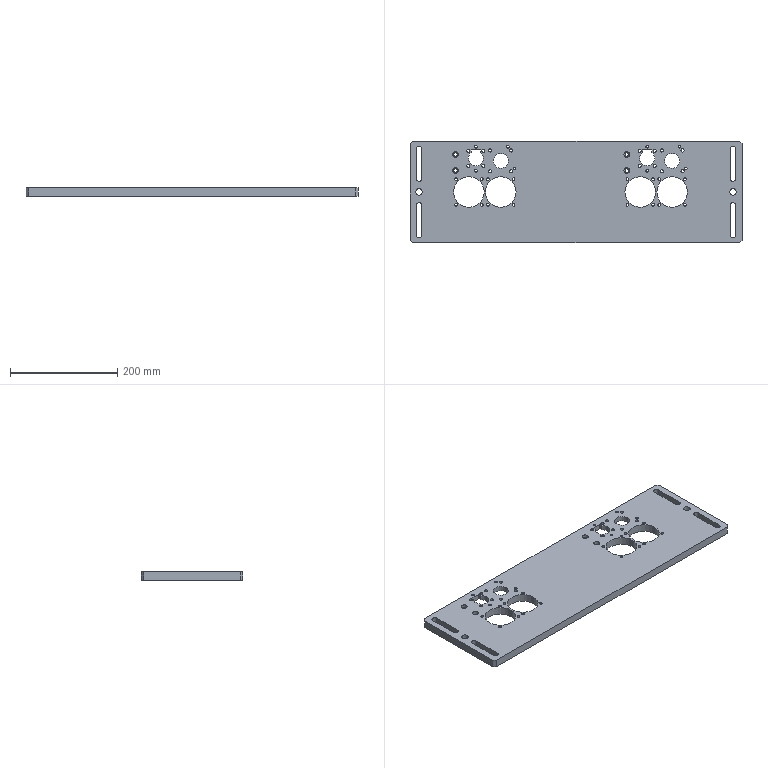Part | SolidWorks | features Cut 4, HoleWzd 4, ICE 2, LPattern 2, Chamfer 1, Extrusion 1, Fillet 1 | 1 solid | 172 faces | box 620 x 190 x 15 mm | volume 1473802 mm3 | cylinder 134 | plane 38 | commonest cylinder face diameters 5 x56 6 x32 28 x10 6.6 x8 10.5 x8 11 x8